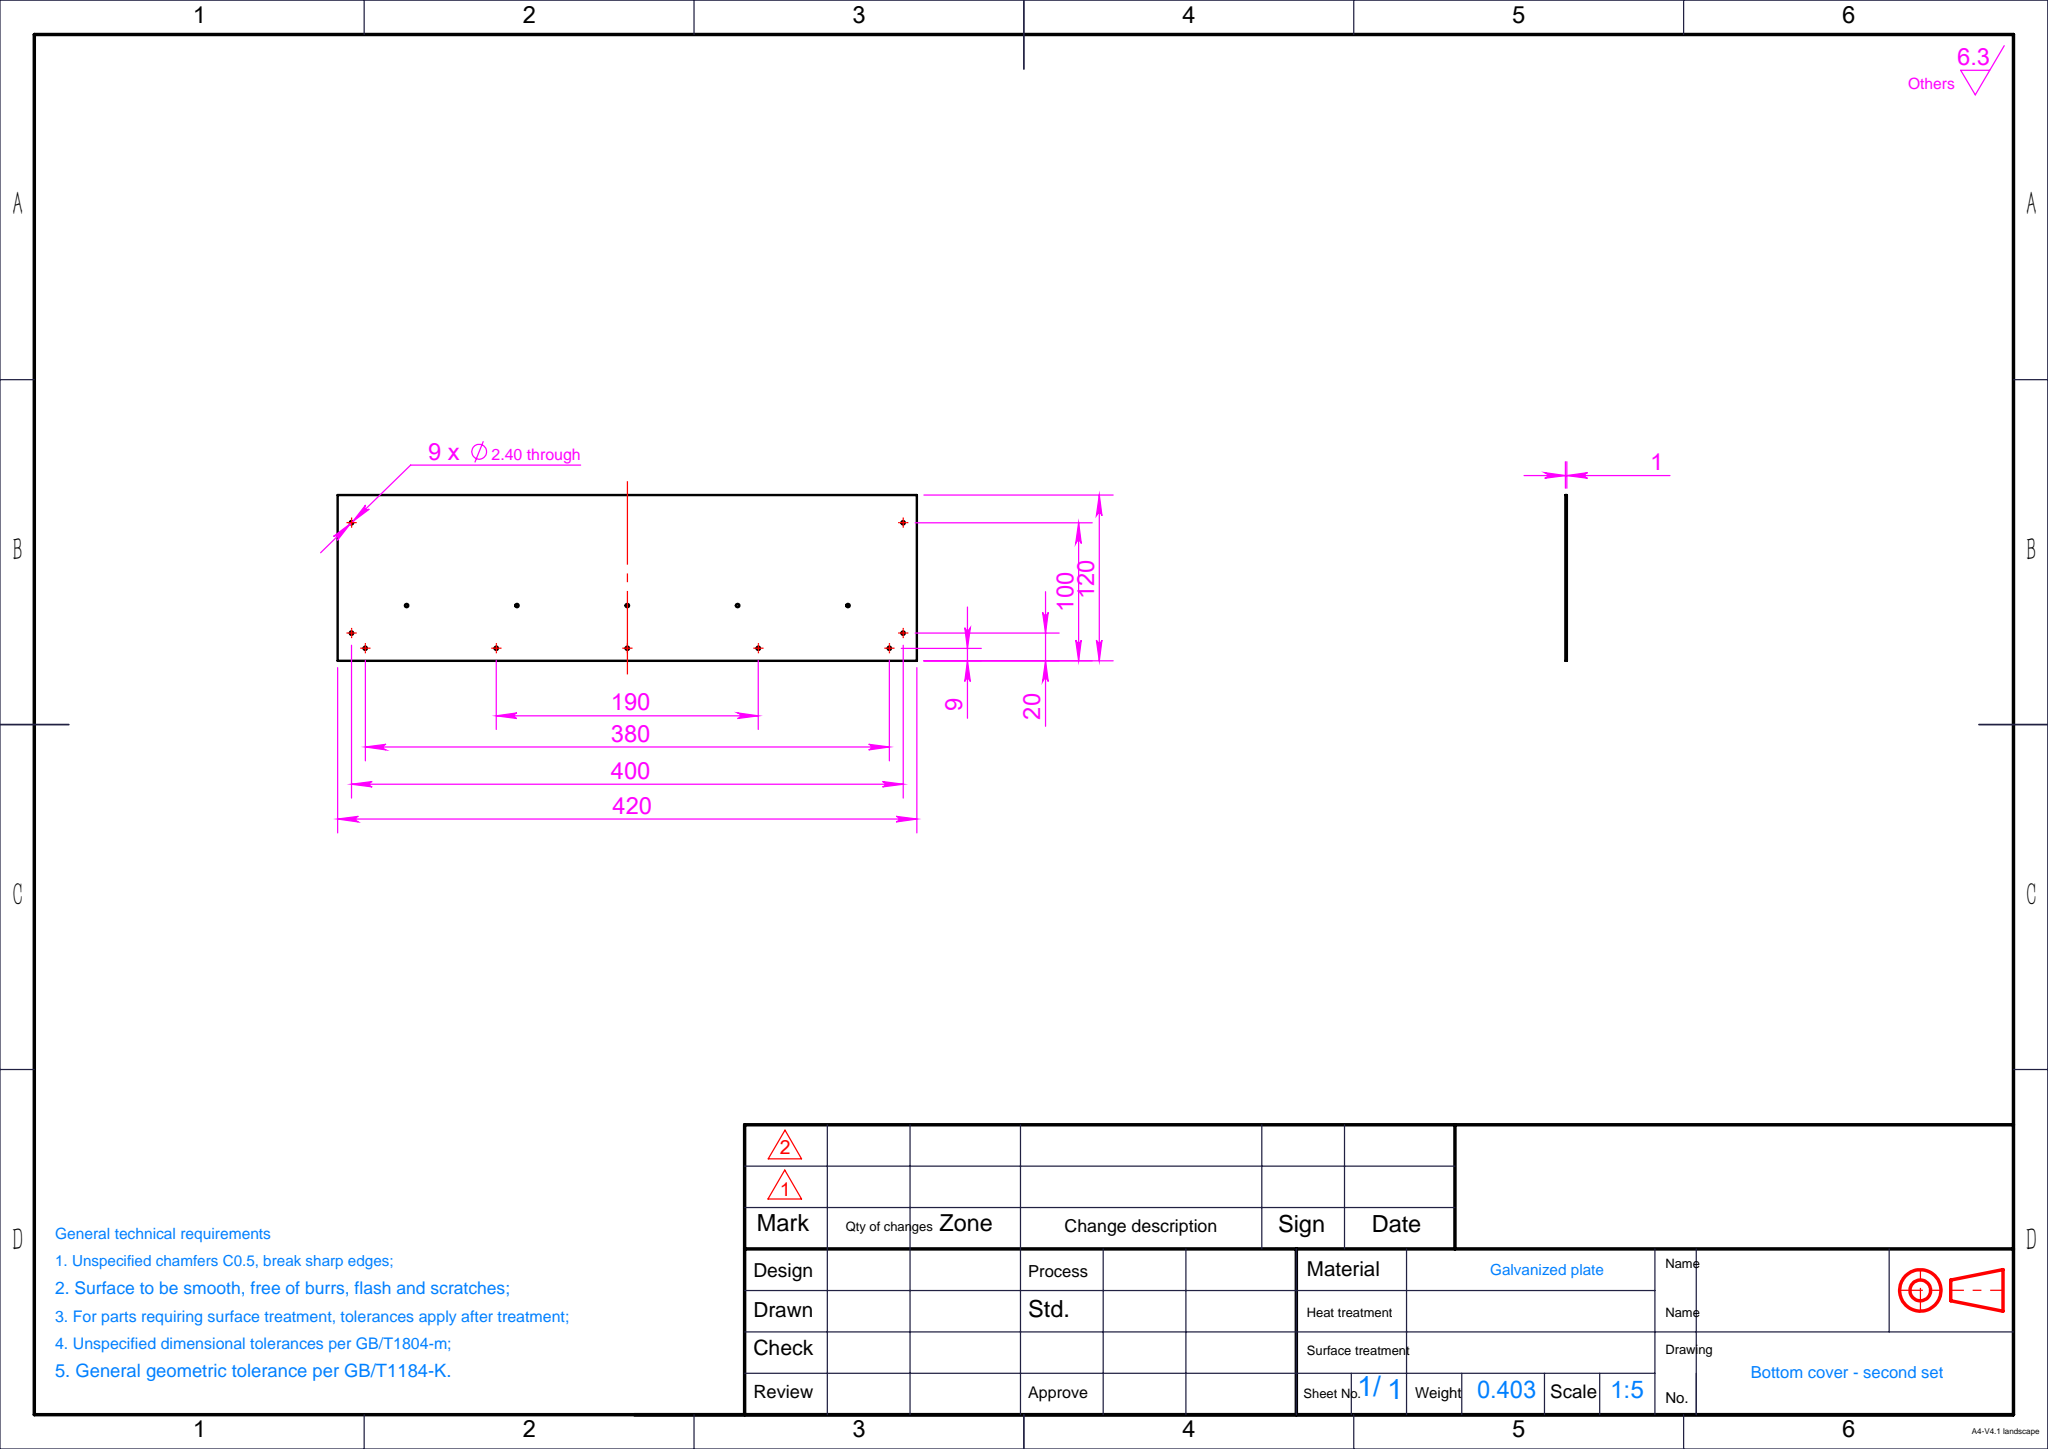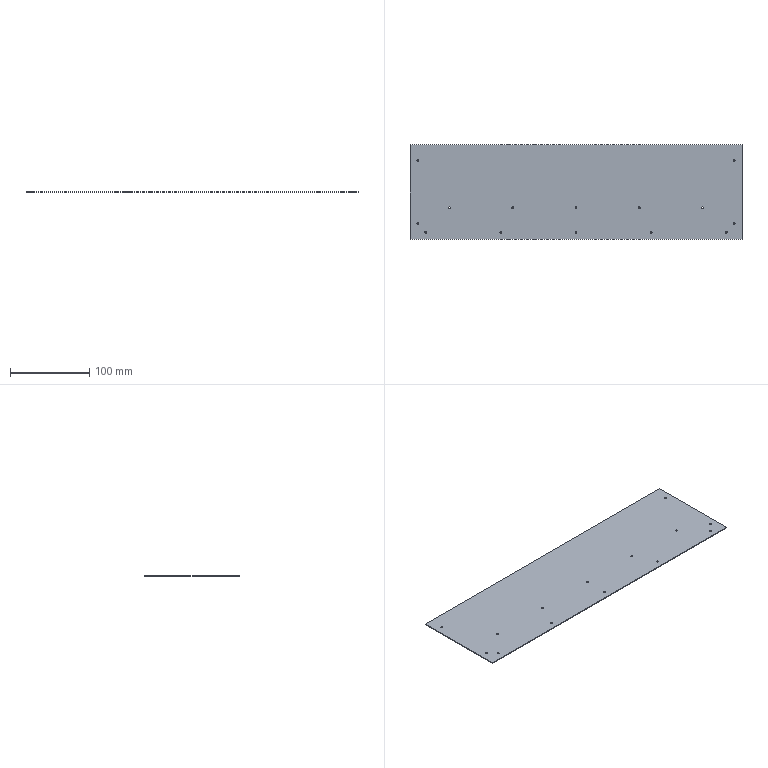Part | SolidWorks | features 3DProfileFeature 1, Chamfer 1, FlatPattern 1, HoleWzd 1, SMBaseFlange 1, SheetMetal 1, SketchPattern 1 | 1 solid | 34 faces | box 420 x 120 x 1 mm | volume 50337 mm3 | cylinder 28 | plane 6 | commonest cylinder face diameters 2.4 x28